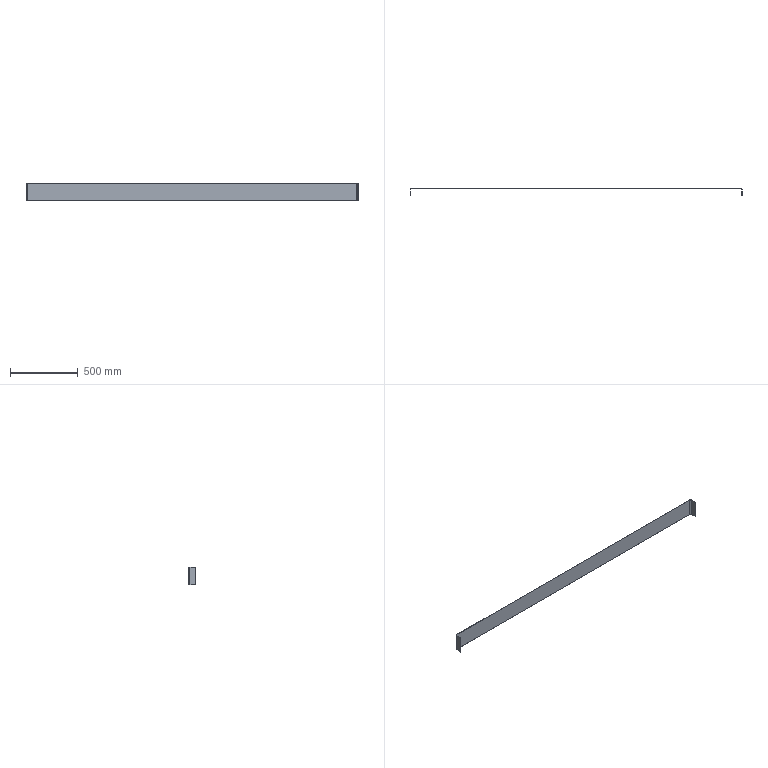Part | SolidWorks | features BaseBody 1 | 1 solid | 14 faces | box 2454 x 50 x 130 mm | volume 330700 mm3 | plane 10 | cylinder 4 | commonest cylinder face diameters 18 x2 20 x2
STEP:
#1=CARTESIAN_POINT('',(-1217.,0.,130.));
#2=VERTEX_POINT('',#1);
#3=CARTESIAN_POINT('',(1217.,0.,130.));
#4=VERTEX_POINT('',#3);
#5=CARTESIAN_POINT('',(-1217.,0.,130.));
#6=DIRECTION('',(1.,0.,0.));
#7=VECTOR('',#6,1000.);
#8=LINE('',#5,#7);
#9=EDGE_CURVE('',#2,#4,#8,.T.);
#10=ORIENTED_EDGE('',*,*,#9,.T.);
#11=CARTESIAN_POINT('',(1217.,0.,0.));
#12=VERTEX_POINT('',#11);
#13=CARTESIAN_POINT('',(1217.,0.,130.));
#14=DIRECTION('',(0.,0.,-1.));
#15=VECTOR('',#14,1000.);
#16=LINE('',#13,#15);
#17=EDGE_CURVE('',#4,#12,#16,.T.);
#18=ORIENTED_EDGE('',*,*,#17,.T.);
#19=CARTESIAN_POINT('',(-1217.,0.,0.));
#20=VERTEX_POINT('',#19);
#21=CARTESIAN_POINT('',(-1217.,0.,0.));
#22=DIRECTION('',(-1.,0.,0.));
#23=VECTOR('',#22,1000.);
#24=LINE('',#21,#23);
#25=EDGE_CURVE('',#12,#20,#24,.T.);
#26=ORIENTED_EDGE('',*,*,#25,.T.);
#27=CARTESIAN_POINT('',(-1217.,0.,130.));
#28=DIRECTION('',(0.,0.,1.));
#29=VECTOR('',#28,1000.);
#30=LINE('',#27,#29);
#31=EDGE_CURVE('',#20,#2,#30,.T.);
#32=ORIENTED_EDGE('',*,*,#31,.T.);
#33=EDGE_LOOP('',(#10,#18,#26,#32));
#34=FACE_OUTER_BOUND('',#33,.T.);
#35=CARTESIAN_POINT('',(-1217.,0.,130.));
#36=DIRECTION('',(0.,1.,0.));
#37=DIRECTION('',(-1.,0.,0.));
#38=AXIS2_PLACEMENT_3D('',#35,#36,#37);
#39=PLANE('',#38);
#40=ADVANCED_FACE('',(#34),#39,.T.);
#41=CARTESIAN_POINT('',(1227.,-10.,130.));
#42=VERTEX_POINT('',#41);
#43=CARTESIAN_POINT('',(1217.,-10.,130.));
#44=DIRECTION('',(0.,0.,-1.));
#45=DIRECTION('',(-1.,0.,0.));
#46=AXIS2_PLACEMENT_3D('',#43,#44,#45);
#47=CIRCLE('',#46,10.);
#48=EDGE_CURVE('',#4,#42,#47,.T.);
#49=ORIENTED_EDGE('',*,*,#48,.T.);
#50=CARTESIAN_POINT('',(1227.,-10.,0.));
#51=VERTEX_POINT('',#50);
#52=CARTESIAN_POINT('',(1227.,-10.,130.));
#53=DIRECTION('',(0.,0.,-1.));
#54=VECTOR('',#53,1000.);
#55=LINE('',#52,#54);
#56=EDGE_CURVE('',#42,#51,#55,.T.);
#57=ORIENTED_EDGE('',*,*,#56,.T.);
#58=CARTESIAN_POINT('',(1217.,-10.,0.));
#59=DIRECTION('',(0.,0.,1.));
#60=DIRECTION('',(-1.,0.,0.));
#61=AXIS2_PLACEMENT_3D('',#58,#59,#60);
#62=CIRCLE('',#61,10.);
#63=EDGE_CURVE('',#51,#12,#62,.T.);
#64=ORIENTED_EDGE('',*,*,#63,.T.);
#65=ORIENTED_EDGE('',*,*,#17,.F.);
#66=EDGE_LOOP('',(#49,#57,#64,#65));
#67=FACE_OUTER_BOUND('',#66,.T.);
#68=CARTESIAN_POINT('',(1217.,-10.,130.));
#69=DIRECTION('',(0.,0.,-1.));
#70=DIRECTION('',(-1.,0.,0.));
#71=AXIS2_PLACEMENT_3D('',#68,#69,#70);
#72=CYLINDRICAL_SURFACE('',#71,10.);
#73=ADVANCED_FACE('',(#67),#72,.T.);
#74=CARTESIAN_POINT('',(1227.,-50.,130.));
#75=VERTEX_POINT('',#74);
#76=CARTESIAN_POINT('',(1226.,-50.,130.));
#77=VERTEX_POINT('',#76);
#78=CARTESIAN_POINT('',(1227.,-50.,130.));
#79=DIRECTION('',(-1.,0.,0.));
#80=VECTOR('',#79,1000.);
#81=LINE('',#78,#80);
#82=EDGE_CURVE('',#75,#77,#81,.T.);
#83=ORIENTED_EDGE('',*,*,#82,.F.);
#84=CARTESIAN_POINT('',(1227.,-10.,130.));
#85=DIRECTION('',(0.,-1.,0.));
#86=VECTOR('',#85,1000.);
#87=LINE('',#84,#86);
#88=EDGE_CURVE('',#42,#75,#87,.T.);
#89=ORIENTED_EDGE('',*,*,#88,.F.);
#90=ORIENTED_EDGE('',*,*,#48,.F.);
#91=ORIENTED_EDGE('',*,*,#9,.F.);
#92=CARTESIAN_POINT('',(-1227.,-10.,130.));
#93=VERTEX_POINT('',#92);
#94=CARTESIAN_POINT('',(-1217.,-10.,130.));
#95=DIRECTION('',(0.,0.,-1.));
#96=DIRECTION('',(-1.,0.,0.));
#97=AXIS2_PLACEMENT_3D('',#94,#95,#96);
#98=CIRCLE('',#97,10.);
#99=EDGE_CURVE('',#93,#2,#98,.T.);
#100=ORIENTED_EDGE('',*,*,#99,.F.);
#101=CARTESIAN_POINT('',(-1227.,-50.,130.));
#102=VERTEX_POINT('',#101);
#103=CARTESIAN_POINT('',(-1227.,-10.,130.));
#104=DIRECTION('',(0.,1.,0.));
#105=VECTOR('',#104,1000.);
#106=LINE('',#103,#105);
#107=EDGE_CURVE('',#102,#93,#106,.T.);
#108=ORIENTED_EDGE('',*,*,#107,.F.);
#109=CARTESIAN_POINT('',(-1226.,-50.,130.));
#110=VERTEX_POINT('',#109);
#111=CARTESIAN_POINT('',(-1226.,-50.,130.));
#112=DIRECTION('',(-1.,0.,0.));
#113=VECTOR('',#112,1000.);
#114=LINE('',#111,#113);
#115=EDGE_CURVE('',#110,#102,#114,.T.);
#116=ORIENTED_EDGE('',*,*,#115,.F.);
#117=CARTESIAN_POINT('',(-1226.,-10.,130.));
#118=VERTEX_POINT('',#117);
#119=CARTESIAN_POINT('',(-1226.,-10.,130.));
#120=DIRECTION('',(0.,-1.,0.));
#121=VECTOR('',#120,1000.);
#122=LINE('',#119,#121);
#123=EDGE_CURVE('',#118,#110,#122,.T.);
#124=ORIENTED_EDGE('',*,*,#123,.F.);
#125=CARTESIAN_POINT('',(-1217.,-1.,130.));
#126=VERTEX_POINT('',#125);
#127=CARTESIAN_POINT('',(-1217.,-10.,130.));
#128=DIRECTION('',(0.,0.,1.));
#129=DIRECTION('',(-1.,0.,0.));
#130=AXIS2_PLACEMENT_3D('',#127,#128,#129);
#131=CIRCLE('',#130,9.);
#132=EDGE_CURVE('',#126,#118,#131,.T.);
#133=ORIENTED_EDGE('',*,*,#132,.F.);
#134=CARTESIAN_POINT('',(1217.,-1.,130.));
#135=VERTEX_POINT('',#134);
#136=CARTESIAN_POINT('',(1217.,-1.,130.));
#137=DIRECTION('',(-1.,0.,0.));
#138=VECTOR('',#137,1000.);
#139=LINE('',#136,#138);
#140=EDGE_CURVE('',#135,#126,#139,.T.);
#141=ORIENTED_EDGE('',*,*,#140,.F.);
#142=CARTESIAN_POINT('',(1226.,-10.,130.));
#143=VERTEX_POINT('',#142);
#144=CARTESIAN_POINT('',(1217.,-10.,130.));
#145=DIRECTION('',(0.,0.,1.));
#146=DIRECTION('',(-1.,0.,0.));
#147=AXIS2_PLACEMENT_3D('',#144,#145,#146);
#148=CIRCLE('',#147,9.);
#149=EDGE_CURVE('',#143,#135,#148,.T.);
#150=ORIENTED_EDGE('',*,*,#149,.F.);
#151=CARTESIAN_POINT('',(1226.,-10.,130.));
#152=DIRECTION('',(0.,1.,0.));
#153=VECTOR('',#152,1000.);
#154=LINE('',#151,#153);
#155=EDGE_CURVE('',#77,#143,#154,.T.);
#156=ORIENTED_EDGE('',*,*,#155,.F.);
#157=EDGE_LOOP('',(#83,#89,#90,#91,#100,#108,#116,#124,#133,#141,#150,#156));
#158=FACE_OUTER_BOUND('',#157,.T.);
#159=CARTESIAN_POINT('',(1217.,-10.,130.));
#160=DIRECTION('',(0.,0.,-1.));
#161=DIRECTION('',(-1.,0.,0.));
#162=AXIS2_PLACEMENT_3D('',#159,#160,#161);
#163=PLANE('',#162);
#164=ADVANCED_FACE('',(#158),#163,.F.);
#165=ORIENTED_EDGE('',*,*,#99,.T.);
#166=ORIENTED_EDGE('',*,*,#31,.F.);
#167=CARTESIAN_POINT('',(-1227.,-10.,0.));
#168=VERTEX_POINT('',#167);
#169=CARTESIAN_POINT('',(-1217.,-10.,0.));
#170=DIRECTION('',(0.,0.,1.));
#171=DIRECTION('',(-1.,0.,0.));
#172=AXIS2_PLACEMENT_3D('',#169,#170,#171);
#173=CIRCLE('',#172,10.);
#174=EDGE_CURVE('',#20,#168,#173,.T.);
#175=ORIENTED_EDGE('',*,*,#174,.T.);
#176=CARTESIAN_POINT('',(-1227.,-10.,130.));
#177=DIRECTION('',(0.,0.,1.));
#178=VECTOR('',#177,1000.);
#179=LINE('',#176,#178);
#180=EDGE_CURVE('',#168,#93,#179,.T.);
#181=ORIENTED_EDGE('',*,*,#180,.T.);
#182=EDGE_LOOP('',(#165,#166,#175,#181));
#183=FACE_OUTER_BOUND('',#182,.T.);
#184=CARTESIAN_POINT('',(-1217.,-10.,130.));
#185=DIRECTION('',(0.,0.,-1.));
#186=DIRECTION('',(-1.,0.,0.));
#187=AXIS2_PLACEMENT_3D('',#184,#185,#186);
#188=CYLINDRICAL_SURFACE('',#187,10.);
#189=ADVANCED_FACE('',(#183),#188,.T.);
#190=CARTESIAN_POINT('',(1227.,-50.,0.));
#191=VERTEX_POINT('',#190);
#192=CARTESIAN_POINT('',(1227.,-10.,0.));
#193=DIRECTION('',(0.,-1.,0.));
#194=VECTOR('',#193,1000.);
#195=LINE('',#192,#194);
#196=EDGE_CURVE('',#51,#191,#195,.T.);
#197=ORIENTED_EDGE('',*,*,#196,.T.);
#198=CARTESIAN_POINT('',(1226.,-50.,0.));
#199=VERTEX_POINT('',#198);
#200=CARTESIAN_POINT('',(1227.,-50.,0.));
#201=DIRECTION('',(1.,0.,0.));
#202=VECTOR('',#201,1000.);
#203=LINE('',#200,#202);
#204=EDGE_CURVE('',#199,#191,#203,.T.);
#205=ORIENTED_EDGE('',*,*,#204,.F.);
#206=CARTESIAN_POINT('',(1226.,-10.,0.));
#207=VERTEX_POINT('',#206);
#208=CARTESIAN_POINT('',(1226.,-10.,0.));
#209=DIRECTION('',(0.,1.,0.));
#210=VECTOR('',#209,1000.);
#211=LINE('',#208,#210);
#212=EDGE_CURVE('',#199,#207,#211,.T.);
#213=ORIENTED_EDGE('',*,*,#212,.T.);
#214=CARTESIAN_POINT('',(1217.,-1.,0.));
#215=VERTEX_POINT('',#214);
#216=CARTESIAN_POINT('',(1217.,-10.,0.));
#217=DIRECTION('',(0.,0.,1.));
#218=DIRECTION('',(-1.,0.,0.));
#219=AXIS2_PLACEMENT_3D('',#216,#217,#218);
#220=CIRCLE('',#219,9.);
#221=EDGE_CURVE('',#207,#215,#220,.T.);
#222=ORIENTED_EDGE('',*,*,#221,.T.);
#223=CARTESIAN_POINT('',(-1217.,-1.,0.));
#224=VERTEX_POINT('',#223);
#225=CARTESIAN_POINT('',(1217.,-1.,0.));
#226=DIRECTION('',(-1.,0.,0.));
#227=VECTOR('',#226,1000.);
#228=LINE('',#225,#227);
#229=EDGE_CURVE('',#215,#224,#228,.T.);
#230=ORIENTED_EDGE('',*,*,#229,.T.);
#231=CARTESIAN_POINT('',(-1226.,-10.,0.));
#232=VERTEX_POINT('',#231);
#233=CARTESIAN_POINT('',(-1217.,-10.,0.));
#234=DIRECTION('',(0.,0.,1.));
#235=DIRECTION('',(-1.,0.,0.));
#236=AXIS2_PLACEMENT_3D('',#233,#234,#235);
#237=CIRCLE('',#236,9.);
#238=EDGE_CURVE('',#224,#232,#237,.T.);
#239=ORIENTED_EDGE('',*,*,#238,.T.);
#240=CARTESIAN_POINT('',(-1226.,-50.,0.));
#241=VERTEX_POINT('',#240);
#242=CARTESIAN_POINT('',(-1226.,-10.,0.));
#243=DIRECTION('',(0.,-1.,0.));
#244=VECTOR('',#243,1000.);
#245=LINE('',#242,#244);
#246=EDGE_CURVE('',#232,#241,#245,.T.);
#247=ORIENTED_EDGE('',*,*,#246,.T.);
#248=CARTESIAN_POINT('',(-1227.,-50.,0.));
#249=VERTEX_POINT('',#248);
#250=CARTESIAN_POINT('',(-1226.,-50.,0.));
#251=DIRECTION('',(1.,0.,0.));
#252=VECTOR('',#251,1000.);
#253=LINE('',#250,#252);
#254=EDGE_CURVE('',#249,#241,#253,.T.);
#255=ORIENTED_EDGE('',*,*,#254,.F.);
#256=CARTESIAN_POINT('',(-1227.,-10.,0.));
#257=DIRECTION('',(0.,1.,0.));
#258=VECTOR('',#257,1000.);
#259=LINE('',#256,#258);
#260=EDGE_CURVE('',#249,#168,#259,.T.);
#261=ORIENTED_EDGE('',*,*,#260,.T.);
#262=ORIENTED_EDGE('',*,*,#174,.F.);
#263=ORIENTED_EDGE('',*,*,#25,.F.);
#264=ORIENTED_EDGE('',*,*,#63,.F.);
#265=EDGE_LOOP('',(#197,#205,#213,#222,#230,#239,#247,#255,#261,#262,#263,#264));
#266=FACE_OUTER_BOUND('',#265,.T.);
#267=CARTESIAN_POINT('',(1217.,-10.,0.));
#268=DIRECTION('',(0.,0.,-1.));
#269=DIRECTION('',(-1.,0.,0.));
#270=AXIS2_PLACEMENT_3D('',#267,#268,#269);
#271=PLANE('',#270);
#272=ADVANCED_FACE('',(#266),#271,.T.);
#273=ORIENTED_EDGE('',*,*,#88,.T.);
#274=CARTESIAN_POINT('',(1227.,-50.,130.));
#275=DIRECTION('',(0.,0.,-1.));
#276=VECTOR('',#275,1000.);
#277=LINE('',#274,#276);
#278=EDGE_CURVE('',#75,#191,#277,.T.);
#279=ORIENTED_EDGE('',*,*,#278,.T.);
#280=ORIENTED_EDGE('',*,*,#196,.F.);
#281=ORIENTED_EDGE('',*,*,#56,.F.);
#282=EDGE_LOOP('',(#273,#279,#280,#281));
#283=FACE_OUTER_BOUND('',#282,.T.);
#284=CARTESIAN_POINT('',(1227.,-10.,130.));
#285=DIRECTION('',(1.,0.,0.));
#286=DIRECTION('',(0.,0.,-1.));
#287=AXIS2_PLACEMENT_3D('',#284,#285,#286);
#288=PLANE('',#287);
#289=ADVANCED_FACE('',(#283),#288,.T.);
#290=CARTESIAN_POINT('',(1226.,-50.,130.));
#291=DIRECTION('',(0.,0.,-1.));
#292=VECTOR('',#291,1000.);
#293=LINE('',#290,#292);
#294=EDGE_CURVE('',#77,#199,#293,.T.);
#295=ORIENTED_EDGE('',*,*,#294,.F.);
#296=ORIENTED_EDGE('',*,*,#155,.T.);
#297=CARTESIAN_POINT('',(1226.,-10.,130.));
#298=DIRECTION('',(0.,0.,1.));
#299=VECTOR('',#298,1000.);
#300=LINE('',#297,#299);
#301=EDGE_CURVE('',#207,#143,#300,.T.);
#302=ORIENTED_EDGE('',*,*,#301,.F.);
#303=ORIENTED_EDGE('',*,*,#212,.F.);
#304=EDGE_LOOP('',(#295,#296,#302,#303));
#305=FACE_OUTER_BOUND('',#304,.T.);
#306=CARTESIAN_POINT('',(1226.,-10.,130.));
#307=DIRECTION('',(1.,0.,0.));
#308=DIRECTION('',(0.,0.,-1.));
#309=AXIS2_PLACEMENT_3D('',#306,#307,#308);
#310=PLANE('',#309);
#311=ADVANCED_FACE('',(#305),#310,.F.);
#312=ORIENTED_EDGE('',*,*,#107,.T.);
#313=ORIENTED_EDGE('',*,*,#180,.F.);
#314=ORIENTED_EDGE('',*,*,#260,.F.);
#315=CARTESIAN_POINT('',(-1227.,-50.,130.));
#316=DIRECTION('',(0.,0.,1.));
#317=VECTOR('',#316,1000.);
#318=LINE('',#315,#317);
#319=EDGE_CURVE('',#249,#102,#318,.T.);
#320=ORIENTED_EDGE('',*,*,#319,.T.);
#321=EDGE_LOOP('',(#312,#313,#314,#320));
#322=FACE_OUTER_BOUND('',#321,.T.);
#323=CARTESIAN_POINT('',(-1227.,-10.,130.));
#324=DIRECTION('',(-1.,0.,0.));
#325=DIRECTION('',(0.,0.,1.));
#326=AXIS2_PLACEMENT_3D('',#323,#324,#325);
#327=PLANE('',#326);
#328=ADVANCED_FACE('',(#322),#327,.T.);
#329=CARTESIAN_POINT('',(-1226.,-10.,130.));
#330=DIRECTION('',(0.,0.,-1.));
#331=VECTOR('',#330,1000.);
#332=LINE('',#329,#331);
#333=EDGE_CURVE('',#118,#232,#332,.T.);
#334=ORIENTED_EDGE('',*,*,#333,.F.);
#335=ORIENTED_EDGE('',*,*,#123,.T.);
#336=CARTESIAN_POINT('',(-1226.,-50.,130.));
#337=DIRECTION('',(0.,0.,1.));
#338=VECTOR('',#337,1000.);
#339=LINE('',#336,#338);
#340=EDGE_CURVE('',#241,#110,#339,.T.);
#341=ORIENTED_EDGE('',*,*,#340,.F.);
#342=ORIENTED_EDGE('',*,*,#246,.F.);
#343=EDGE_LOOP('',(#334,#335,#341,#342));
#344=FACE_OUTER_BOUND('',#343,.T.);
#345=CARTESIAN_POINT('',(-1226.,-10.,130.));
#346=DIRECTION('',(-1.,0.,0.));
#347=DIRECTION('',(0.,0.,1.));
#348=AXIS2_PLACEMENT_3D('',#345,#346,#347);
#349=PLANE('',#348);
#350=ADVANCED_FACE('',(#344),#349,.F.);
#351=CARTESIAN_POINT('',(-1217.,-1.,130.));
#352=DIRECTION('',(0.,0.,-1.));
#353=VECTOR('',#352,1000.);
#354=LINE('',#351,#353);
#355=EDGE_CURVE('',#126,#224,#354,.T.);
#356=ORIENTED_EDGE('',*,*,#355,.F.);
#357=ORIENTED_EDGE('',*,*,#132,.T.);
#358=ORIENTED_EDGE('',*,*,#333,.T.);
#359=ORIENTED_EDGE('',*,*,#238,.F.);
#360=EDGE_LOOP('',(#356,#357,#358,#359));
#361=FACE_OUTER_BOUND('',#360,.T.);
#362=CARTESIAN_POINT('',(-1217.,-10.,130.));
#363=DIRECTION('',(0.,0.,-1.));
#364=DIRECTION('',(-1.,0.,0.));
#365=AXIS2_PLACEMENT_3D('',#362,#363,#364);
#366=CYLINDRICAL_SURFACE('',#365,9.);
#367=ADVANCED_FACE('',(#361),#366,.F.);
#368=CARTESIAN_POINT('',(1217.,-1.,130.));
#369=DIRECTION('',(0.,0.,-1.));
#370=VECTOR('',#369,1000.);
#371=LINE('',#368,#370);
#372=EDGE_CURVE('',#135,#215,#371,.T.);
#373=ORIENTED_EDGE('',*,*,#372,.F.);
#374=ORIENTED_EDGE('',*,*,#140,.T.);
#375=ORIENTED_EDGE('',*,*,#355,.T.);
#376=ORIENTED_EDGE('',*,*,#229,.F.);
#377=EDGE_LOOP('',(#373,#374,#375,#376));
#378=FACE_OUTER_BOUND('',#377,.T.);
#379=CARTESIAN_POINT('',(-1217.,-1.,130.));
#380=DIRECTION('',(0.,1.,0.));
#381=DIRECTION('',(-1.,0.,0.));
#382=AXIS2_PLACEMENT_3D('',#379,#380,#381);
#383=PLANE('',#382);
#384=ADVANCED_FACE('',(#378),#383,.F.);
#385=ORIENTED_EDGE('',*,*,#301,.T.);
#386=ORIENTED_EDGE('',*,*,#149,.T.);
#387=ORIENTED_EDGE('',*,*,#372,.T.);
#388=ORIENTED_EDGE('',*,*,#221,.F.);
#389=EDGE_LOOP('',(#385,#386,#387,#388));
#390=FACE_OUTER_BOUND('',#389,.T.);
#391=CARTESIAN_POINT('',(1217.,-10.,130.));
#392=DIRECTION('',(0.,0.,-1.));
#393=DIRECTION('',(-1.,0.,0.));
#394=AXIS2_PLACEMENT_3D('',#391,#392,#393);
#395=CYLINDRICAL_SURFACE('',#394,9.);
#396=ADVANCED_FACE('',(#390),#395,.F.);
#397=ORIENTED_EDGE('',*,*,#82,.T.);
#398=ORIENTED_EDGE('',*,*,#294,.T.);
#399=ORIENTED_EDGE('',*,*,#204,.T.);
#400=ORIENTED_EDGE('',*,*,#278,.F.);
#401=EDGE_LOOP('',(#397,#398,#399,#400));
#402=FACE_OUTER_BOUND('',#401,.T.);
#403=CARTESIAN_POINT('',(1227.,-50.,130.));
#404=DIRECTION('',(0.,-1.,0.));
#405=DIRECTION('',(0.,0.,-1.));
#406=AXIS2_PLACEMENT_3D('',#403,#404,#405);
#407=PLANE('',#406);
#408=ADVANCED_FACE('',(#402),#407,.T.);
#409=ORIENTED_EDGE('',*,*,#115,.T.);
#410=ORIENTED_EDGE('',*,*,#319,.F.);
#411=ORIENTED_EDGE('',*,*,#254,.T.);
#412=ORIENTED_EDGE('',*,*,#340,.T.);
#413=EDGE_LOOP('',(#409,#410,#411,#412));
#414=FACE_OUTER_BOUND('',#413,.T.);
#415=CARTESIAN_POINT('',(-1226.,-50.,130.));
#416=DIRECTION('',(0.,-1.,0.));
#417=DIRECTION('',(0.,0.,-1.));
#418=AXIS2_PLACEMENT_3D('',#415,#416,#417);
#419=PLANE('',#418);
#420=ADVANCED_FACE('',(#414),#419,.T.);
#421=CLOSED_SHELL('',(#40,#73,#164,#189,#272,#289,#311,#328,#350,#367,#384,#396,#408,#420));
#422=MANIFOLD_SOLID_BREP('',#421);
#423=CARTESIAN_POINT('',(0.,0.,0.));
#424=DIRECTION('',(0.,0.,1.));
#425=DIRECTION('',(1.,0.,0.));
#426=AXIS2_PLACEMENT_3D('',#423,#424,#425);
#427=(LENGTH_UNIT()NAMED_UNIT(*)SI_UNIT(.MILLI.,.METRE.));
#428=UNCERTAINTY_MEASURE_WITH_UNIT(LENGTH_MEASURE(0.00001),#427,'','');
#429=(NAMED_UNIT(*)PLANE_ANGLE_UNIT()SI_UNIT($,.RADIAN.));
#430=(NAMED_UNIT(*)SI_UNIT($,.STERADIAN.)SOLID_ANGLE_UNIT());
#431=(GEOMETRIC_REPRESENTATION_CONTEXT(3)GLOBAL_UNCERTAINTY_ASSIGNED_CONTEXT((#428))GLOBAL_UNIT_ASSIGNED_CONTEXT((#427,#429,#430))REPRESENTATION_CONTEXT('',''));
#432=ADVANCED_BREP_SHAPE_REPRESENTATION('',(#422,#426),#431);